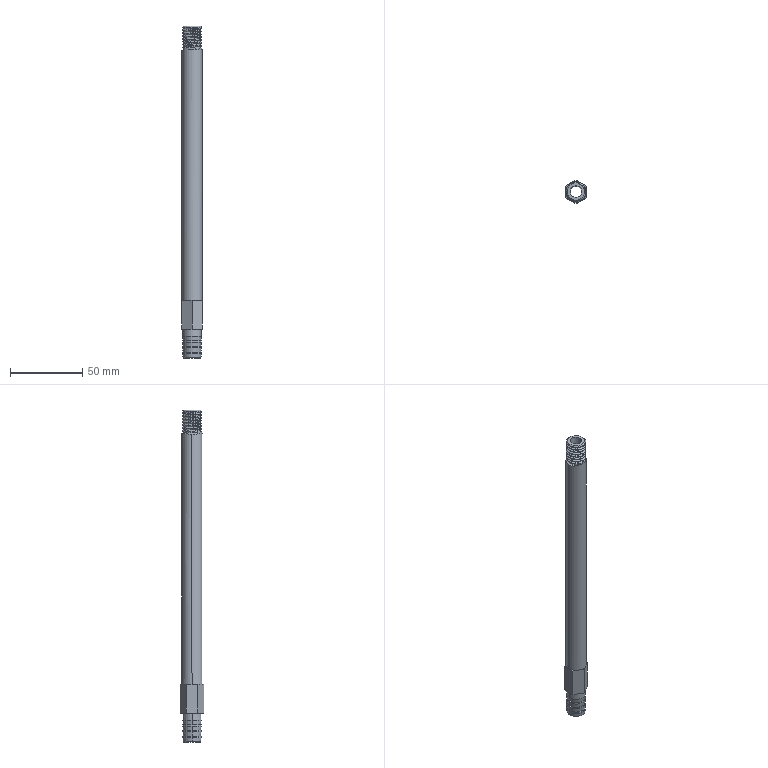Part | SolidWorks | features BaseBody 1 | 1 solid | 82 faces | box 14 x 16.166 x 230 mm | volume 23150 mm3 | cylinder 45 | plane 21 | cone 14 | spline 2 | commonest cylinder face diameters 13.6 x17 11.6 x16 13 x8 8 x2 14 x2